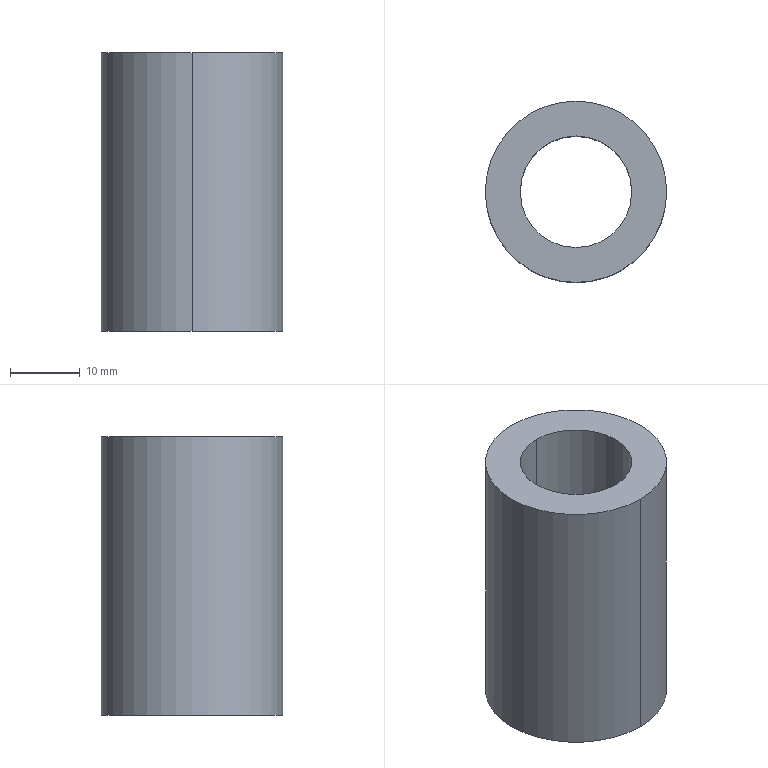Part | SolidWorks | features BaseBody 1 | 1 solid | 6 faces | box 26 x 26 x 40 mm | volume 13195 mm3 | cylinder 4 | plane 2 | commonest cylinder face diameters 16 x2 26 x2
STEP:
#1=CARTESIAN_POINT('',(-276.782,70.138,20.));
#2=VERTEX_POINT('',#1);
#3=CARTESIAN_POINT('',(-276.782,54.138,20.));
#4=VERTEX_POINT('',#3);
#5=CARTESIAN_POINT('',(-276.782,62.138,20.));
#6=DIRECTION('',(0.,0.,1.));
#7=DIRECTION('',(0.,-1.,0.));
#8=AXIS2_PLACEMENT_3D('',#5,#6,#7);
#9=CIRCLE('',#8,8.);
#10=EDGE_CURVE('',#2,#4,#9,.T.);
#11=ORIENTED_EDGE('',*,*,#10,.T.);
#12=CARTESIAN_POINT('',(-276.782,54.138,-20.));
#13=VERTEX_POINT('',#12);
#14=CARTESIAN_POINT('',(-276.782,54.138,20.));
#15=DIRECTION('',(0.,0.,-1.));
#16=VECTOR('',#15,1000.);
#17=LINE('',#14,#16);
#18=EDGE_CURVE('',#4,#13,#17,.T.);
#19=ORIENTED_EDGE('',*,*,#18,.T.);
#20=CARTESIAN_POINT('',(-276.782,70.138,-20.));
#21=VERTEX_POINT('',#20);
#22=CARTESIAN_POINT('',(-276.782,62.138,-20.));
#23=DIRECTION('',(0.,0.,1.));
#24=DIRECTION('',(0.,-1.,0.));
#25=AXIS2_PLACEMENT_3D('',#22,#23,#24);
#26=CIRCLE('',#25,8.);
#27=EDGE_CURVE('',#21,#13,#26,.T.);
#28=ORIENTED_EDGE('',*,*,#27,.F.);
#29=CARTESIAN_POINT('',(-276.782,70.138,20.));
#30=DIRECTION('',(0.,0.,-1.));
#31=VECTOR('',#30,1000.);
#32=LINE('',#29,#31);
#33=EDGE_CURVE('',#2,#21,#32,.T.);
#34=ORIENTED_EDGE('',*,*,#33,.F.);
#35=EDGE_LOOP('',(#11,#19,#28,#34));
#36=FACE_OUTER_BOUND('',#35,.T.);
#37=CARTESIAN_POINT('',(-276.782,62.138,20.));
#38=DIRECTION('',(0.,0.,-1.));
#39=DIRECTION('',(0.,1.,0.));
#40=AXIS2_PLACEMENT_3D('',#37,#38,#39);
#41=CYLINDRICAL_SURFACE('',#40,8.);
#42=ADVANCED_FACE('',(#36),#41,.F.);
#43=CARTESIAN_POINT('',(-276.782,49.138,20.));
#44=VERTEX_POINT('',#43);
#45=CARTESIAN_POINT('',(-276.782,75.138,20.));
#46=VERTEX_POINT('',#45);
#47=CARTESIAN_POINT('',(-276.782,62.138,20.));
#48=DIRECTION('',(0.,0.,1.));
#49=DIRECTION('',(0.,-1.,0.));
#50=AXIS2_PLACEMENT_3D('',#47,#48,#49);
#51=CIRCLE('',#50,13.);
#52=EDGE_CURVE('',#44,#46,#51,.T.);
#53=ORIENTED_EDGE('',*,*,#52,.F.);
#54=CARTESIAN_POINT('',(-276.782,49.138,-20.));
#55=VERTEX_POINT('',#54);
#56=CARTESIAN_POINT('',(-276.782,49.138,20.));
#57=DIRECTION('',(0.,0.,-1.));
#58=VECTOR('',#57,1000.);
#59=LINE('',#56,#58);
#60=EDGE_CURVE('',#44,#55,#59,.T.);
#61=ORIENTED_EDGE('',*,*,#60,.T.);
#62=CARTESIAN_POINT('',(-276.782,75.138,-20.));
#63=VERTEX_POINT('',#62);
#64=CARTESIAN_POINT('',(-276.782,62.138,-20.));
#65=DIRECTION('',(0.,0.,1.));
#66=DIRECTION('',(0.,-1.,0.));
#67=AXIS2_PLACEMENT_3D('',#64,#65,#66);
#68=CIRCLE('',#67,13.);
#69=EDGE_CURVE('',#55,#63,#68,.T.);
#70=ORIENTED_EDGE('',*,*,#69,.T.);
#71=CARTESIAN_POINT('',(-276.782,75.138,20.));
#72=DIRECTION('',(0.,0.,-1.));
#73=VECTOR('',#72,1000.);
#74=LINE('',#71,#73);
#75=EDGE_CURVE('',#46,#63,#74,.T.);
#76=ORIENTED_EDGE('',*,*,#75,.F.);
#77=EDGE_LOOP('',(#53,#61,#70,#76));
#78=FACE_OUTER_BOUND('',#77,.T.);
#79=CARTESIAN_POINT('',(-276.782,62.138,20.));
#80=DIRECTION('',(0.,0.,-1.));
#81=DIRECTION('',(0.,1.,0.));
#82=AXIS2_PLACEMENT_3D('',#79,#80,#81);
#83=CYLINDRICAL_SURFACE('',#82,13.);
#84=ADVANCED_FACE('',(#78),#83,.T.);
#85=CARTESIAN_POINT('',(-276.782,62.138,20.));
#86=DIRECTION('',(0.,0.,1.));
#87=DIRECTION('',(0.,-1.,0.));
#88=AXIS2_PLACEMENT_3D('',#85,#86,#87);
#89=CIRCLE('',#88,13.);
#90=EDGE_CURVE('',#46,#44,#89,.T.);
#91=ORIENTED_EDGE('',*,*,#90,.T.);
#92=ORIENTED_EDGE('',*,*,#52,.T.);
#93=EDGE_LOOP('',(#91,#92));
#94=FACE_OUTER_BOUND('',#93,.T.);
#95=ORIENTED_EDGE('',*,*,#10,.F.);
#96=CARTESIAN_POINT('',(-276.782,62.138,20.));
#97=DIRECTION('',(0.,0.,1.));
#98=DIRECTION('',(0.,-1.,0.));
#99=AXIS2_PLACEMENT_3D('',#96,#97,#98);
#100=CIRCLE('',#99,8.);
#101=EDGE_CURVE('',#4,#2,#100,.T.);
#102=ORIENTED_EDGE('',*,*,#101,.F.);
#103=EDGE_LOOP('',(#95,#102));
#104=FACE_BOUND('',#103,.T.);
#105=CARTESIAN_POINT('',(-276.782,62.138,20.));
#106=DIRECTION('',(0.,0.,1.));
#107=DIRECTION('',(0.,-1.,0.));
#108=AXIS2_PLACEMENT_3D('',#105,#106,#107);
#109=PLANE('',#108);
#110=ADVANCED_FACE('',(#94,#104),#109,.T.);
#111=CARTESIAN_POINT('',(-276.782,62.138,-20.));
#112=DIRECTION('',(0.,0.,1.));
#113=DIRECTION('',(0.,-1.,0.));
#114=AXIS2_PLACEMENT_3D('',#111,#112,#113);
#115=CIRCLE('',#114,13.);
#116=EDGE_CURVE('',#63,#55,#115,.T.);
#117=ORIENTED_EDGE('',*,*,#116,.F.);
#118=ORIENTED_EDGE('',*,*,#69,.F.);
#119=EDGE_LOOP('',(#117,#118));
#120=FACE_OUTER_BOUND('',#119,.T.);
#121=ORIENTED_EDGE('',*,*,#27,.T.);
#122=CARTESIAN_POINT('',(-276.782,62.138,-20.));
#123=DIRECTION('',(0.,0.,1.));
#124=DIRECTION('',(0.,-1.,0.));
#125=AXIS2_PLACEMENT_3D('',#122,#123,#124);
#126=CIRCLE('',#125,8.);
#127=EDGE_CURVE('',#13,#21,#126,.T.);
#128=ORIENTED_EDGE('',*,*,#127,.T.);
#129=EDGE_LOOP('',(#121,#128));
#130=FACE_BOUND('',#129,.T.);
#131=CARTESIAN_POINT('',(-276.782,62.138,-20.));
#132=DIRECTION('',(0.,0.,1.));
#133=DIRECTION('',(0.,-1.,0.));
#134=AXIS2_PLACEMENT_3D('',#131,#132,#133);
#135=PLANE('',#134);
#136=ADVANCED_FACE('',(#120,#130),#135,.F.);
#137=ORIENTED_EDGE('',*,*,#60,.F.);
#138=ORIENTED_EDGE('',*,*,#90,.F.);
#139=ORIENTED_EDGE('',*,*,#75,.T.);
#140=ORIENTED_EDGE('',*,*,#116,.T.);
#141=EDGE_LOOP('',(#137,#138,#139,#140));
#142=FACE_OUTER_BOUND('',#141,.T.);
#143=CARTESIAN_POINT('',(-276.782,62.138,20.));
#144=DIRECTION('',(0.,0.,-1.));
#145=DIRECTION('',(0.,1.,0.));
#146=AXIS2_PLACEMENT_3D('',#143,#144,#145);
#147=CYLINDRICAL_SURFACE('',#146,13.);
#148=ADVANCED_FACE('',(#142),#147,.T.);
#149=ORIENTED_EDGE('',*,*,#18,.F.);
#150=ORIENTED_EDGE('',*,*,#101,.T.);
#151=ORIENTED_EDGE('',*,*,#33,.T.);
#152=ORIENTED_EDGE('',*,*,#127,.F.);
#153=EDGE_LOOP('',(#149,#150,#151,#152));
#154=FACE_OUTER_BOUND('',#153,.T.);
#155=CARTESIAN_POINT('',(-276.782,62.138,20.));
#156=DIRECTION('',(0.,0.,-1.));
#157=DIRECTION('',(0.,1.,0.));
#158=AXIS2_PLACEMENT_3D('',#155,#156,#157);
#159=CYLINDRICAL_SURFACE('',#158,8.);
#160=ADVANCED_FACE('',(#154),#159,.F.);
#161=CLOSED_SHELL('',(#42,#84,#110,#136,#148,#160));
#162=MANIFOLD_SOLID_BREP('',#161);
#163=CARTESIAN_POINT('',(0.,0.,0.));
#164=DIRECTION('',(0.,0.,1.));
#165=DIRECTION('',(1.,0.,0.));
#166=AXIS2_PLACEMENT_3D('',#163,#164,#165);
#167=(LENGTH_UNIT()NAMED_UNIT(*)SI_UNIT(.MILLI.,.METRE.));
#168=UNCERTAINTY_MEASURE_WITH_UNIT(LENGTH_MEASURE(0.00001),#167,'','');
#169=(NAMED_UNIT(*)PLANE_ANGLE_UNIT()SI_UNIT($,.RADIAN.));
#170=(NAMED_UNIT(*)SI_UNIT($,.STERADIAN.)SOLID_ANGLE_UNIT());
#171=(GEOMETRIC_REPRESENTATION_CONTEXT(3)GLOBAL_UNCERTAINTY_ASSIGNED_CONTEXT((#168))GLOBAL_UNIT_ASSIGNED_CONTEXT((#167,#169,#170))REPRESENTATION_CONTEXT('',''));
#172=ADVANCED_BREP_SHAPE_REPRESENTATION('',(#162,#166),#171);